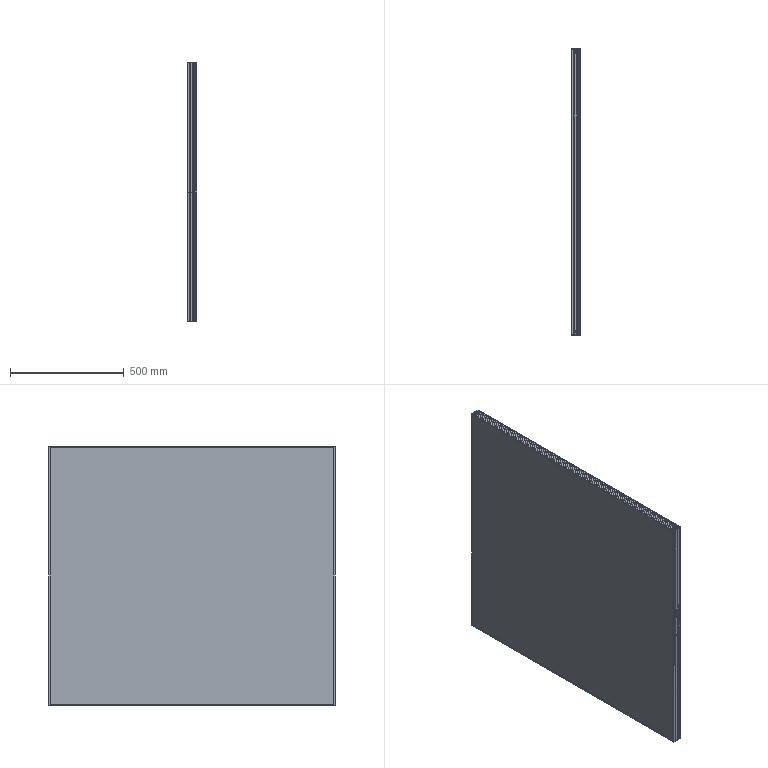Part | SolidWorks | 7 solids | 390 faces | box 40 x 1260 x 1140 mm | volume 17028562 mm3 | plane 254 | cylinder 136 | commonest cylinder face diameters 0.6 x80 4 x32 3 x16 5 x8